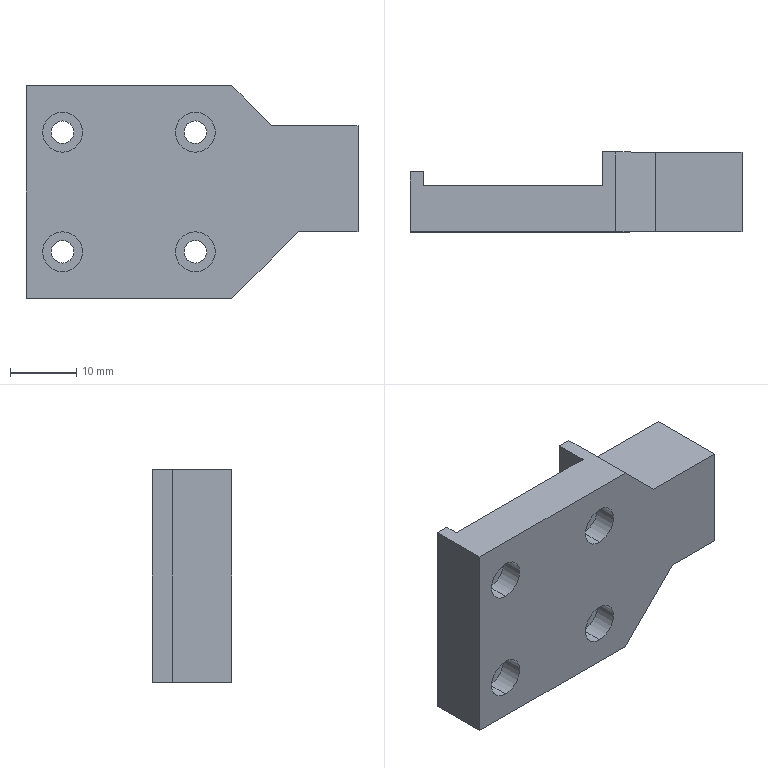Part | STEP file | PN_0016 | 1 solid | 42 faces | box 50 x 12 x 32 mm | volume 11255 mm3 | cylinder 20 | plane 18 | cone 4 | commonest cylinder face diameters 3.4 x8 6 x8 2.5 x4